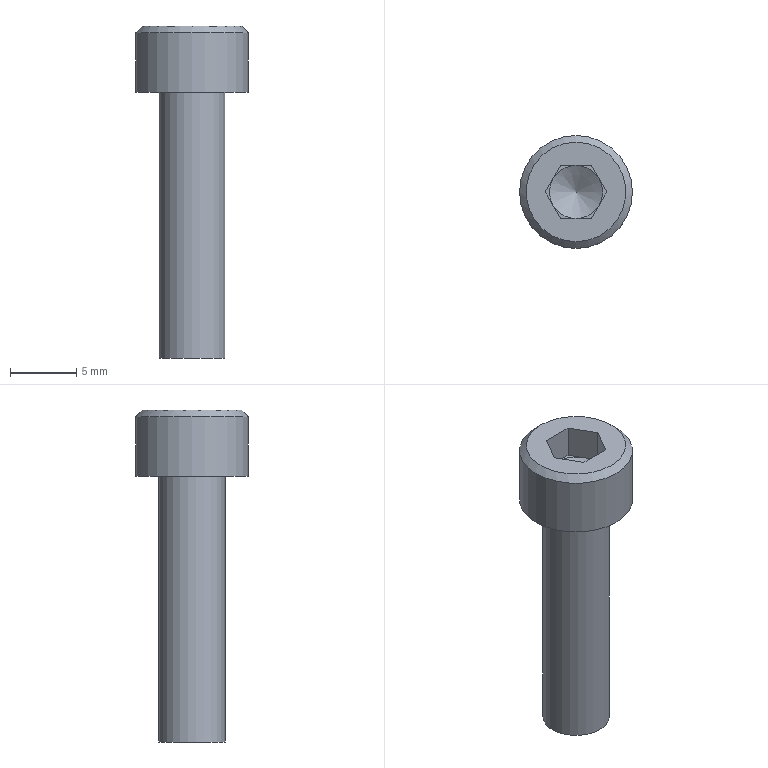Part | NX | features 5003_322_CB5-20 2 | 1 solid | 19 faces | box 8.5 x 8.5 x 25 mm | volume 633.542 mm3 | plane 15 | cylinder 2 | cone 2 | commonest cylinder face diameters 5 x1 8.5 x1
STEP:
#1=CARTESIAN_POINT('',(26.025,-50.75,-228.7));
#2=VERTEX_POINT('',#1);
#3=CARTESIAN_POINT('',(26.025,-47.,-228.7));
#4=DIRECTION('',(0.,0.,-1.));
#5=DIRECTION('',(0.,-1.,0.));
#6=AXIS2_PLACEMENT_3D('',#3,#4,#5);
#7=CIRCLE('',#6,3.75);
#8=EDGE_CURVE('',#2,#2,#7,.F.);
#9=ORIENTED_EDGE('',*,*,#8,.T.);
#10=EDGE_LOOP('',(#9));
#11=FACE_BOUND('',#10,.T.);
#12=CARTESIAN_POINT('',(28.334,-47.,-228.7));
#13=VERTEX_POINT('',#12);
#14=CARTESIAN_POINT('',(27.18,-45.,-228.7));
#15=VERTEX_POINT('',#14);
#16=CARTESIAN_POINT('',(28.334,-47.,-228.7));
#17=DIRECTION('',(-0.5,0.866,0.));
#18=VECTOR('',#17,1000.);
#19=LINE('',#16,#18);
#20=EDGE_CURVE('',#13,#15,#19,.T.);
#21=ORIENTED_EDGE('',*,*,#20,.F.);
#22=CARTESIAN_POINT('',(27.18,-49.,-228.7));
#23=VERTEX_POINT('',#22);
#24=CARTESIAN_POINT('',(27.18,-49.,-228.7));
#25=DIRECTION('',(0.5,0.866,0.));
#26=VECTOR('',#25,1000.);
#27=LINE('',#24,#26);
#28=EDGE_CURVE('',#23,#13,#27,.T.);
#29=ORIENTED_EDGE('',*,*,#28,.F.);
#30=CARTESIAN_POINT('',(24.87,-49.,-228.7));
#31=VERTEX_POINT('',#30);
#32=CARTESIAN_POINT('',(24.87,-49.,-228.7));
#33=DIRECTION('',(1.,0.,0.));
#34=VECTOR('',#33,1000.);
#35=LINE('',#32,#34);
#36=EDGE_CURVE('',#31,#23,#35,.T.);
#37=ORIENTED_EDGE('',*,*,#36,.F.);
#38=CARTESIAN_POINT('',(23.716,-47.,-228.7));
#39=VERTEX_POINT('',#38);
#40=CARTESIAN_POINT('',(23.716,-47.,-228.7));
#41=DIRECTION('',(0.5,-0.866,0.));
#42=VECTOR('',#41,1000.);
#43=LINE('',#40,#42);
#44=EDGE_CURVE('',#39,#31,#43,.T.);
#45=ORIENTED_EDGE('',*,*,#44,.F.);
#46=CARTESIAN_POINT('',(24.87,-45.,-228.7));
#47=VERTEX_POINT('',#46);
#48=CARTESIAN_POINT('',(24.87,-45.,-228.7));
#49=DIRECTION('',(-0.5,-0.866,0.));
#50=VECTOR('',#49,1000.);
#51=LINE('',#48,#50);
#52=EDGE_CURVE('',#47,#39,#51,.T.);
#53=ORIENTED_EDGE('',*,*,#52,.F.);
#54=CARTESIAN_POINT('',(27.18,-45.,-228.7));
#55=DIRECTION('',(-1.,0.,0.));
#56=VECTOR('',#55,1000.);
#57=LINE('',#54,#56);
#58=EDGE_CURVE('',#15,#47,#57,.T.);
#59=ORIENTED_EDGE('',*,*,#58,.F.);
#60=EDGE_LOOP('',(#21,#29,#37,#45,#53,#59));
#61=FACE_BOUND('',#60,.T.);
#62=CARTESIAN_POINT('',(21.775,-47.,-228.7));
#63=DIRECTION('',(0.,0.,-1.));
#64=DIRECTION('',(0.,-1.,0.));
#65=AXIS2_PLACEMENT_3D('',#62,#63,#64);
#66=PLANE('',#65);
#67=ADVANCED_FACE('',(#11,#61),#66,.F.);
#68=CARTESIAN_POINT('',(26.025,-44.5,-253.7));
#69=VERTEX_POINT('',#68);
#70=CARTESIAN_POINT('',(26.025,-47.,-253.7));
#71=DIRECTION('',(0.,0.,1.));
#72=DIRECTION('',(0.,1.,0.));
#73=AXIS2_PLACEMENT_3D('',#70,#71,#72);
#74=CIRCLE('',#73,2.5);
#75=EDGE_CURVE('',#69,#69,#74,.T.);
#76=ORIENTED_EDGE('',*,*,#75,.F.);
#77=EDGE_LOOP('',(#76));
#78=FACE_BOUND('',#77,.T.);
#79=CARTESIAN_POINT('',(26.025,-47.,-253.7));
#80=DIRECTION('',(0.,0.,1.));
#81=DIRECTION('',(0.,1.,0.));
#82=AXIS2_PLACEMENT_3D('',#79,#80,#81);
#83=PLANE('',#82);
#84=ADVANCED_FACE('',(#78),#83,.F.);
#85=CARTESIAN_POINT('',(26.025,-44.5,-233.7));
#86=VERTEX_POINT('',#85);
#87=CARTESIAN_POINT('',(26.025,-47.,-233.7));
#88=DIRECTION('',(0.,0.,1.));
#89=DIRECTION('',(0.,1.,0.));
#90=AXIS2_PLACEMENT_3D('',#87,#88,#89);
#91=CIRCLE('',#90,2.5);
#92=EDGE_CURVE('',#86,#86,#91,.T.);
#93=ORIENTED_EDGE('',*,*,#92,.F.);
#94=EDGE_LOOP('',(#93));
#95=FACE_BOUND('',#94,.T.);
#96=ORIENTED_EDGE('',*,*,#75,.T.);
#97=EDGE_LOOP('',(#96));
#98=FACE_BOUND('',#97,.T.);
#99=CARTESIAN_POINT('',(26.025,-47.,-228.7));
#100=DIRECTION('',(0.,0.,1.));
#101=DIRECTION('',(0.,1.,0.));
#102=AXIS2_PLACEMENT_3D('',#99,#100,#101);
#103=CYLINDRICAL_SURFACE('',#102,2.5);
#104=ADVANCED_FACE('',(#95,#98),#103,.T.);
#105=CARTESIAN_POINT('',(26.025,-42.75,-233.7));
#106=VERTEX_POINT('',#105);
#107=CARTESIAN_POINT('',(26.025,-47.,-233.7));
#108=DIRECTION('',(0.,0.,1.));
#109=DIRECTION('',(0.,1.,0.));
#110=AXIS2_PLACEMENT_3D('',#107,#108,#109);
#111=CIRCLE('',#110,4.25);
#112=EDGE_CURVE('',#106,#106,#111,.T.);
#113=ORIENTED_EDGE('',*,*,#112,.F.);
#114=EDGE_LOOP('',(#113));
#115=FACE_BOUND('',#114,.T.);
#116=ORIENTED_EDGE('',*,*,#92,.T.);
#117=EDGE_LOOP('',(#116));
#118=FACE_BOUND('',#117,.T.);
#119=CARTESIAN_POINT('',(23.525,-47.,-233.7));
#120=DIRECTION('',(0.,0.,1.));
#121=DIRECTION('',(0.,1.,0.));
#122=AXIS2_PLACEMENT_3D('',#119,#120,#121);
#123=PLANE('',#122);
#124=ADVANCED_FACE('',(#115,#118),#123,.F.);
#125=CARTESIAN_POINT('',(26.025,-51.25,-229.2));
#126=VERTEX_POINT('',#125);
#127=CARTESIAN_POINT('',(26.025,-47.,-229.2));
#128=DIRECTION('',(0.,0.,-1.));
#129=DIRECTION('',(0.,-1.,0.));
#130=AXIS2_PLACEMENT_3D('',#127,#128,#129);
#131=CIRCLE('',#130,4.25);
#132=EDGE_CURVE('',#126,#126,#131,.T.);
#133=ORIENTED_EDGE('',*,*,#132,.T.);
#134=EDGE_LOOP('',(#133));
#135=FACE_BOUND('',#134,.T.);
#136=ORIENTED_EDGE('',*,*,#112,.T.);
#137=EDGE_LOOP('',(#136));
#138=FACE_BOUND('',#137,.T.);
#139=CARTESIAN_POINT('',(26.025,-47.,-228.7));
#140=DIRECTION('',(0.,0.,1.));
#141=DIRECTION('',(0.,1.,0.));
#142=AXIS2_PLACEMENT_3D('',#139,#140,#141);
#143=CYLINDRICAL_SURFACE('',#142,4.25);
#144=ADVANCED_FACE('',(#135,#138),#143,.T.);
#145=ORIENTED_EDGE('',*,*,#132,.F.);
#146=EDGE_LOOP('',(#145));
#147=FACE_BOUND('',#146,.T.);
#148=ORIENTED_EDGE('',*,*,#8,.F.);
#149=EDGE_LOOP('',(#148));
#150=FACE_BOUND('',#149,.T.);
#151=CARTESIAN_POINT('',(26.025,-47.,-228.7));
#152=DIRECTION('',(0.,0.,-1.));
#153=DIRECTION('',(0.,-1.,0.));
#154=AXIS2_PLACEMENT_3D('',#151,#152,#153);
#155=CONICAL_SURFACE('',#154,3.75,0.7854);
#156=ADVANCED_FACE('',(#147,#150),#155,.T.);
#157=CARTESIAN_POINT('',(27.18,-49.,-231.2));
#158=VERTEX_POINT('',#157);
#159=CARTESIAN_POINT('',(27.757,-48.,-231.2));
#160=VERTEX_POINT('',#159);
#161=CARTESIAN_POINT('',(27.18,-49.,-231.2));
#162=DIRECTION('',(0.5,0.866,0.));
#163=VECTOR('',#162,1000.);
#164=LINE('',#161,#163);
#165=EDGE_CURVE('',#158,#160,#164,.T.);
#166=ORIENTED_EDGE('',*,*,#165,.F.);
#167=CARTESIAN_POINT('',(27.18,-49.,-231.2));
#168=DIRECTION('',(0.,0.,1.));
#169=VECTOR('',#168,1000.);
#170=LINE('',#167,#169);
#171=EDGE_CURVE('',#158,#23,#170,.T.);
#172=ORIENTED_EDGE('',*,*,#171,.T.);
#173=ORIENTED_EDGE('',*,*,#28,.T.);
#174=CARTESIAN_POINT('',(28.334,-47.,-231.2));
#175=VERTEX_POINT('',#174);
#176=CARTESIAN_POINT('',(28.334,-47.,-231.2));
#177=DIRECTION('',(0.,0.,1.));
#178=VECTOR('',#177,1000.);
#179=LINE('',#176,#178);
#180=EDGE_CURVE('',#175,#13,#179,.T.);
#181=ORIENTED_EDGE('',*,*,#180,.F.);
#182=CARTESIAN_POINT('',(27.18,-49.,-231.2));
#183=DIRECTION('',(0.5,0.866,0.));
#184=VECTOR('',#183,1000.);
#185=LINE('',#182,#184);
#186=EDGE_CURVE('',#160,#175,#185,.T.);
#187=ORIENTED_EDGE('',*,*,#186,.F.);
#188=EDGE_LOOP('',(#166,#172,#173,#181,#187));
#189=FACE_BOUND('',#188,.T.);
#190=CARTESIAN_POINT('',(27.18,-49.,-231.2));
#191=DIRECTION('',(0.866,-0.5,0.));
#192=DIRECTION('',(-0.5,-0.866,0.));
#193=AXIS2_PLACEMENT_3D('',#190,#191,#192);
#194=PLANE('',#193);
#195=ADVANCED_FACE('',(#189),#194,.F.);
#196=CARTESIAN_POINT('',(24.87,-49.,-231.2));
#197=VERTEX_POINT('',#196);
#198=CARTESIAN_POINT('',(26.025,-49.,-231.2));
#199=VERTEX_POINT('',#198);
#200=CARTESIAN_POINT('',(24.87,-49.,-231.2));
#201=DIRECTION('',(1.,0.,0.));
#202=VECTOR('',#201,1000.);
#203=LINE('',#200,#202);
#204=EDGE_CURVE('',#197,#199,#203,.T.);
#205=ORIENTED_EDGE('',*,*,#204,.F.);
#206=CARTESIAN_POINT('',(24.87,-49.,-231.2));
#207=DIRECTION('',(0.,0.,1.));
#208=VECTOR('',#207,1000.);
#209=LINE('',#206,#208);
#210=EDGE_CURVE('',#197,#31,#209,.T.);
#211=ORIENTED_EDGE('',*,*,#210,.T.);
#212=ORIENTED_EDGE('',*,*,#36,.T.);
#213=ORIENTED_EDGE('',*,*,#171,.F.);
#214=CARTESIAN_POINT('',(24.87,-49.,-231.2));
#215=DIRECTION('',(1.,0.,0.));
#216=VECTOR('',#215,1000.);
#217=LINE('',#214,#216);
#218=EDGE_CURVE('',#199,#158,#217,.T.);
#219=ORIENTED_EDGE('',*,*,#218,.F.);
#220=EDGE_LOOP('',(#205,#211,#212,#213,#219));
#221=FACE_BOUND('',#220,.T.);
#222=CARTESIAN_POINT('',(24.87,-49.,-231.2));
#223=DIRECTION('',(0.,-1.,0.));
#224=DIRECTION('',(0.,0.,1.));
#225=AXIS2_PLACEMENT_3D('',#222,#223,#224);
#226=PLANE('',#225);
#227=ADVANCED_FACE('',(#221),#226,.F.);
#228=CARTESIAN_POINT('',(23.716,-47.,-231.2));
#229=VERTEX_POINT('',#228);
#230=CARTESIAN_POINT('',(24.293,-48.,-231.2));
#231=VERTEX_POINT('',#230);
#232=CARTESIAN_POINT('',(23.716,-47.,-231.2));
#233=DIRECTION('',(0.5,-0.866,0.));
#234=VECTOR('',#233,1000.);
#235=LINE('',#232,#234);
#236=EDGE_CURVE('',#229,#231,#235,.T.);
#237=ORIENTED_EDGE('',*,*,#236,.F.);
#238=CARTESIAN_POINT('',(23.716,-47.,-231.2));
#239=DIRECTION('',(0.,0.,1.));
#240=VECTOR('',#239,1000.);
#241=LINE('',#238,#240);
#242=EDGE_CURVE('',#229,#39,#241,.T.);
#243=ORIENTED_EDGE('',*,*,#242,.T.);
#244=ORIENTED_EDGE('',*,*,#44,.T.);
#245=ORIENTED_EDGE('',*,*,#210,.F.);
#246=CARTESIAN_POINT('',(23.716,-47.,-231.2));
#247=DIRECTION('',(0.5,-0.866,0.));
#248=VECTOR('',#247,1000.);
#249=LINE('',#246,#248);
#250=EDGE_CURVE('',#231,#197,#249,.T.);
#251=ORIENTED_EDGE('',*,*,#250,.F.);
#252=EDGE_LOOP('',(#237,#243,#244,#245,#251));
#253=FACE_BOUND('',#252,.T.);
#254=CARTESIAN_POINT('',(23.716,-47.,-231.2));
#255=DIRECTION('',(-0.866,-0.5,0.));
#256=DIRECTION('',(-0.5,0.866,0.));
#257=AXIS2_PLACEMENT_3D('',#254,#255,#256);
#258=PLANE('',#257);
#259=ADVANCED_FACE('',(#253),#258,.F.);
#260=CARTESIAN_POINT('',(24.87,-45.,-231.2));
#261=VERTEX_POINT('',#260);
#262=CARTESIAN_POINT('',(24.293,-46.,-231.2));
#263=VERTEX_POINT('',#262);
#264=CARTESIAN_POINT('',(24.87,-45.,-231.2));
#265=DIRECTION('',(-0.5,-0.866,0.));
#266=VECTOR('',#265,1000.);
#267=LINE('',#264,#266);
#268=EDGE_CURVE('',#261,#263,#267,.T.);
#269=ORIENTED_EDGE('',*,*,#268,.F.);
#270=CARTESIAN_POINT('',(24.87,-45.,-231.2));
#271=DIRECTION('',(0.,0.,1.));
#272=VECTOR('',#271,1000.);
#273=LINE('',#270,#272);
#274=EDGE_CURVE('',#261,#47,#273,.T.);
#275=ORIENTED_EDGE('',*,*,#274,.T.);
#276=ORIENTED_EDGE('',*,*,#52,.T.);
#277=ORIENTED_EDGE('',*,*,#242,.F.);
#278=CARTESIAN_POINT('',(24.87,-45.,-231.2));
#279=DIRECTION('',(-0.5,-0.866,0.));
#280=VECTOR('',#279,1000.);
#281=LINE('',#278,#280);
#282=EDGE_CURVE('',#263,#229,#281,.T.);
#283=ORIENTED_EDGE('',*,*,#282,.F.);
#284=EDGE_LOOP('',(#269,#275,#276,#277,#283));
#285=FACE_BOUND('',#284,.T.);
#286=CARTESIAN_POINT('',(24.87,-45.,-231.2));
#287=DIRECTION('',(-0.866,0.5,0.));
#288=DIRECTION('',(0.5,0.866,0.));
#289=AXIS2_PLACEMENT_3D('',#286,#287,#288);
#290=PLANE('',#289);
#291=ADVANCED_FACE('',(#285),#290,.F.);
#292=CARTESIAN_POINT('',(27.18,-45.,-231.2));
#293=VERTEX_POINT('',#292);
#294=CARTESIAN_POINT('',(26.025,-45.,-231.2));
#295=VERTEX_POINT('',#294);
#296=CARTESIAN_POINT('',(27.18,-45.,-231.2));
#297=DIRECTION('',(-1.,0.,0.));
#298=VECTOR('',#297,1000.);
#299=LINE('',#296,#298);
#300=EDGE_CURVE('',#293,#295,#299,.T.);
#301=ORIENTED_EDGE('',*,*,#300,.F.);
#302=CARTESIAN_POINT('',(27.18,-45.,-231.2));
#303=DIRECTION('',(0.,0.,1.));
#304=VECTOR('',#303,1000.);
#305=LINE('',#302,#304);
#306=EDGE_CURVE('',#293,#15,#305,.T.);
#307=ORIENTED_EDGE('',*,*,#306,.T.);
#308=ORIENTED_EDGE('',*,*,#58,.T.);
#309=ORIENTED_EDGE('',*,*,#274,.F.);
#310=CARTESIAN_POINT('',(27.18,-45.,-231.2));
#311=DIRECTION('',(-1.,0.,0.));
#312=VECTOR('',#311,1000.);
#313=LINE('',#310,#312);
#314=EDGE_CURVE('',#295,#261,#313,.T.);
#315=ORIENTED_EDGE('',*,*,#314,.F.);
#316=EDGE_LOOP('',(#301,#307,#308,#309,#315));
#317=FACE_BOUND('',#316,.T.);
#318=CARTESIAN_POINT('',(27.18,-45.,-231.2));
#319=DIRECTION('',(0.,1.,0.));
#320=DIRECTION('',(1.,0.,0.));
#321=AXIS2_PLACEMENT_3D('',#318,#319,#320);
#322=PLANE('',#321);
#323=ADVANCED_FACE('',(#317),#322,.F.);
#324=CARTESIAN_POINT('',(27.757,-46.,-231.2));
#325=VERTEX_POINT('',#324);
#326=CARTESIAN_POINT('',(28.334,-47.,-231.2));
#327=DIRECTION('',(-0.5,0.866,0.));
#328=VECTOR('',#327,1000.);
#329=LINE('',#326,#328);
#330=EDGE_CURVE('',#175,#325,#329,.T.);
#331=ORIENTED_EDGE('',*,*,#330,.F.);
#332=ORIENTED_EDGE('',*,*,#180,.T.);
#333=ORIENTED_EDGE('',*,*,#20,.T.);
#334=ORIENTED_EDGE('',*,*,#306,.F.);
#335=CARTESIAN_POINT('',(28.334,-47.,-231.2));
#336=DIRECTION('',(-0.5,0.866,0.));
#337=VECTOR('',#336,1000.);
#338=LINE('',#335,#337);
#339=EDGE_CURVE('',#325,#293,#338,.T.);
#340=ORIENTED_EDGE('',*,*,#339,.F.);
#341=EDGE_LOOP('',(#331,#332,#333,#334,#340));
#342=FACE_BOUND('',#341,.T.);
#343=CARTESIAN_POINT('',(28.334,-47.,-231.2));
#344=DIRECTION('',(0.866,0.5,0.));
#345=DIRECTION('',(0.5,-0.866,0.));
#346=AXIS2_PLACEMENT_3D('',#343,#344,#345);
#347=PLANE('',#346);
#348=ADVANCED_FACE('',(#342),#347,.F.);
#349=ORIENTED_EDGE('',*,*,#314,.T.);
#350=ORIENTED_EDGE('',*,*,#268,.T.);
#351=CARTESIAN_POINT('',(26.025,-47.,-231.2));
#352=DIRECTION('',(0.,0.,1.));
#353=DIRECTION('',(1.,0.,0.));
#354=AXIS2_PLACEMENT_3D('',#351,#352,#353);
#355=CIRCLE('',#354,2.);
#356=EDGE_CURVE('',#295,#263,#355,.T.);
#357=ORIENTED_EDGE('',*,*,#356,.F.);
#358=EDGE_LOOP('',(#349,#350,#357));
#359=FACE_BOUND('',#358,.T.);
#360=CARTESIAN_POINT('',(26.025,-47.,-231.2));
#361=DIRECTION('',(0.,0.,1.));
#362=DIRECTION('',(0.,1.,0.));
#363=AXIS2_PLACEMENT_3D('',#360,#361,#362);
#364=PLANE('',#363);
#365=ADVANCED_FACE('',(#359),#364,.T.);
#366=ORIENTED_EDGE('',*,*,#282,.T.);
#367=ORIENTED_EDGE('',*,*,#236,.T.);
#368=CARTESIAN_POINT('',(26.025,-47.,-231.2));
#369=DIRECTION('',(0.,0.,1.));
#370=DIRECTION('',(1.,0.,0.));
#371=AXIS2_PLACEMENT_3D('',#368,#369,#370);
#372=CIRCLE('',#371,2.);
#373=EDGE_CURVE('',#263,#231,#372,.T.);
#374=ORIENTED_EDGE('',*,*,#373,.F.);
#375=EDGE_LOOP('',(#366,#367,#374));
#376=FACE_BOUND('',#375,.T.);
#377=CARTESIAN_POINT('',(26.025,-47.,-231.2));
#378=DIRECTION('',(0.,0.,1.));
#379=DIRECTION('',(0.,1.,0.));
#380=AXIS2_PLACEMENT_3D('',#377,#378,#379);
#381=PLANE('',#380);
#382=ADVANCED_FACE('',(#376),#381,.T.);
#383=ORIENTED_EDGE('',*,*,#250,.T.);
#384=ORIENTED_EDGE('',*,*,#204,.T.);
#385=CARTESIAN_POINT('',(26.025,-47.,-231.2));
#386=DIRECTION('',(0.,0.,1.));
#387=DIRECTION('',(1.,0.,0.));
#388=AXIS2_PLACEMENT_3D('',#385,#386,#387);
#389=CIRCLE('',#388,2.);
#390=EDGE_CURVE('',#231,#199,#389,.T.);
#391=ORIENTED_EDGE('',*,*,#390,.F.);
#392=EDGE_LOOP('',(#383,#384,#391));
#393=FACE_BOUND('',#392,.T.);
#394=CARTESIAN_POINT('',(26.025,-47.,-231.2));
#395=DIRECTION('',(0.,0.,1.));
#396=DIRECTION('',(0.,1.,0.));
#397=AXIS2_PLACEMENT_3D('',#394,#395,#396);
#398=PLANE('',#397);
#399=ADVANCED_FACE('',(#393),#398,.T.);
#400=ORIENTED_EDGE('',*,*,#218,.T.);
#401=ORIENTED_EDGE('',*,*,#165,.T.);
#402=CARTESIAN_POINT('',(26.025,-47.,-231.2));
#403=DIRECTION('',(0.,0.,1.));
#404=DIRECTION('',(1.,0.,0.));
#405=AXIS2_PLACEMENT_3D('',#402,#403,#404);
#406=CIRCLE('',#405,2.);
#407=EDGE_CURVE('',#199,#160,#406,.T.);
#408=ORIENTED_EDGE('',*,*,#407,.F.);
#409=EDGE_LOOP('',(#400,#401,#408));
#410=FACE_BOUND('',#409,.T.);
#411=CARTESIAN_POINT('',(26.025,-47.,-231.2));
#412=DIRECTION('',(0.,0.,1.));
#413=DIRECTION('',(0.,1.,0.));
#414=AXIS2_PLACEMENT_3D('',#411,#412,#413);
#415=PLANE('',#414);
#416=ADVANCED_FACE('',(#410),#415,.T.);
#417=ORIENTED_EDGE('',*,*,#186,.T.);
#418=ORIENTED_EDGE('',*,*,#330,.T.);
#419=CARTESIAN_POINT('',(26.025,-47.,-231.2));
#420=DIRECTION('',(0.,0.,1.));
#421=DIRECTION('',(1.,0.,0.));
#422=AXIS2_PLACEMENT_3D('',#419,#420,#421);
#423=CIRCLE('',#422,2.);
#424=EDGE_CURVE('',#160,#325,#423,.T.);
#425=ORIENTED_EDGE('',*,*,#424,.F.);
#426=EDGE_LOOP('',(#417,#418,#425));
#427=FACE_BOUND('',#426,.T.);
#428=CARTESIAN_POINT('',(26.025,-47.,-231.2));
#429=DIRECTION('',(0.,0.,1.));
#430=DIRECTION('',(0.,1.,0.));
#431=AXIS2_PLACEMENT_3D('',#428,#429,#430);
#432=PLANE('',#431);
#433=ADVANCED_FACE('',(#427),#432,.T.);
#434=ORIENTED_EDGE('',*,*,#339,.T.);
#435=ORIENTED_EDGE('',*,*,#300,.T.);
#436=CARTESIAN_POINT('',(26.025,-47.,-231.2));
#437=DIRECTION('',(0.,0.,1.));
#438=DIRECTION('',(1.,0.,0.));
#439=AXIS2_PLACEMENT_3D('',#436,#437,#438);
#440=CIRCLE('',#439,2.);
#441=EDGE_CURVE('',#325,#295,#440,.T.);
#442=ORIENTED_EDGE('',*,*,#441,.F.);
#443=EDGE_LOOP('',(#434,#435,#442));
#444=FACE_BOUND('',#443,.T.);
#445=CARTESIAN_POINT('',(26.025,-47.,-231.2));
#446=DIRECTION('',(0.,0.,1.));
#447=DIRECTION('',(0.,1.,0.));
#448=AXIS2_PLACEMENT_3D('',#445,#446,#447);
#449=PLANE('',#448);
#450=ADVANCED_FACE('',(#444),#449,.T.);
#451=ORIENTED_EDGE('',*,*,#441,.T.);
#452=ORIENTED_EDGE('',*,*,#356,.T.);
#453=ORIENTED_EDGE('',*,*,#373,.T.);
#454=ORIENTED_EDGE('',*,*,#390,.T.);
#455=ORIENTED_EDGE('',*,*,#407,.T.);
#456=ORIENTED_EDGE('',*,*,#424,.T.);
#457=EDGE_LOOP('',(#451,#452,#453,#454,#455,#456));
#458=FACE_BOUND('',#457,.T.);
#459=CARTESIAN_POINT('',(26.025,-47.,-232.402));
#460=VERTEX_POINT('',#459);
#461=VERTEX_LOOP('',#460);
#462=FACE_BOUND('',#461,.T.);
#463=CARTESIAN_POINT('',(26.025,-47.,-232.402));
#464=DIRECTION('',(0.,0.,1.));
#465=DIRECTION('',(1.,0.,0.));
#466=AXIS2_PLACEMENT_3D('',#463,#464,#465);
#467=CONICAL_SURFACE('',#466,0.,1.03);
#468=ADVANCED_FACE('',(#458,#462),#467,.F.);
#469=CLOSED_SHELL('',(#67,#84,#104,#124,#144,#156,#195,#227,#259,#291,#323,#348,#365,#382,#399,#416,#433,#450,#468));
#470=MANIFOLD_SOLID_BREP('',#469);
#471=(LENGTH_UNIT()NAMED_UNIT(*)SI_UNIT(.MILLI.,.METRE.));
#472=UNCERTAINTY_MEASURE_WITH_UNIT(LENGTH_MEASURE(0.00001),#471,'','');
#473=(NAMED_UNIT(*)PLANE_ANGLE_UNIT()SI_UNIT($,.RADIAN.));
#474=(NAMED_UNIT(*)SI_UNIT($,.STERADIAN.)SOLID_ANGLE_UNIT());
#475=(GEOMETRIC_REPRESENTATION_CONTEXT(3)GLOBAL_UNCERTAINTY_ASSIGNED_CONTEXT((#472))GLOBAL_UNIT_ASSIGNED_CONTEXT((#471,#473,#474))REPRESENTATION_CONTEXT('',''));
#476=ADVANCED_BREP_SHAPE_REPRESENTATION('',(#470),#475);